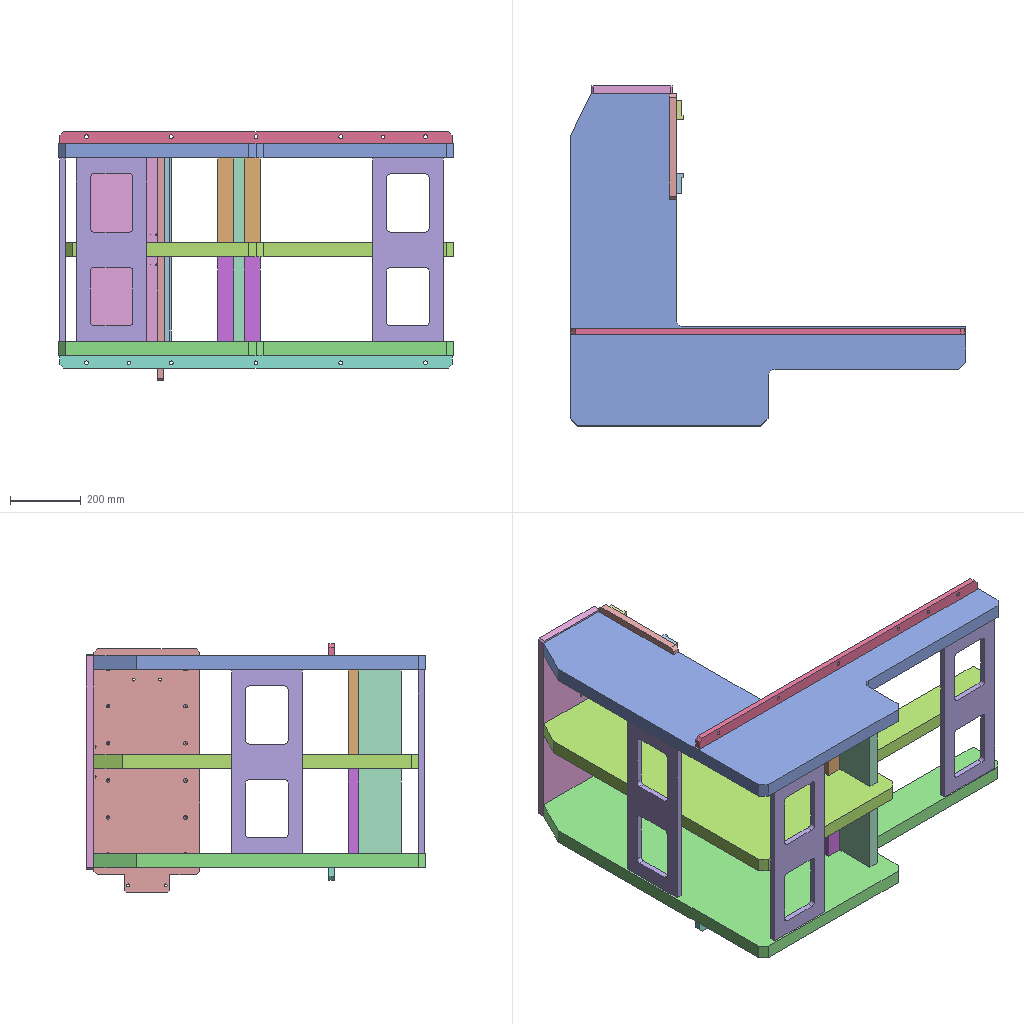Assembly | SolidWorks | 9 different items | 16 placed | box 1120 x 962 x 705 mm
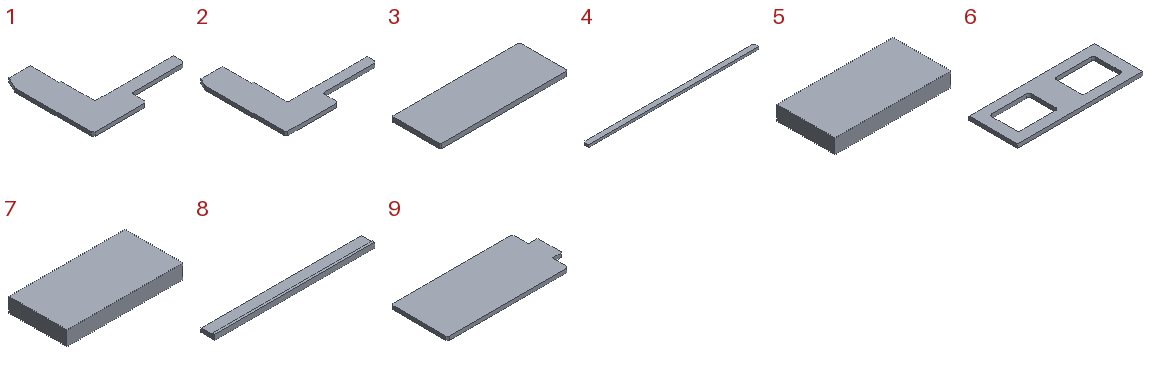Parts list (item | quantity | size | volume | features):
1 | x2 | 1120 x 940 x 40 mm | 16478867 mm3 | features Chamfer 1, Extrusion 1, Fillet 1
2 | x1 | 1099 x 919 x 40 mm | 14868507 mm3 | features Chamfer 1, Extrusion 1, Fillet 1
3 | x1 | 610 x 230 x 22 mm | 3085500 mm3 | features Chamfer 1, Extrusion 1
4 | x2 | 1110 x 35 x 16 mm | 620000 mm3 | features Chamfer 1, Extrusion 1
5 | x2 | 240 x 120 x 30 mm | 864000 mm3 | features Extrusion 1
6 | x3 | 520 x 200 x 16 mm | 1033147 mm3 | features Extrusion 1
7 | x2 | 240 x 120 x 30 mm | 864000 mm3 | features Extrusion 1
8 | x2 | 630 x 55 x 20 mm | 551250 mm3 | features Extrusion 1
9 | x1 | 690 x 300 x 20 mm | 3963509 mm3 | features Chamfer 2, Extrusion 1, Fillet 1
Mates (type | each side: item.copy, entity, surface, feature):
DistanceDim | 1.1 face plane | 2.1 face plane | 2 times
DistanceDim | 2.1 face plane | 1.2 face plane | 2 times
Coincident | 2.1 face plane | 6.1 face plane Boss-Extrude1
Coincident | 1.2 face plane | 6.1 face plane Boss-Extrude1
DistanceDim | 6.1 face plane Boss-Extrude1 | 1.2 face plane
Coincident | 6.1 face plane Boss-Extrude1 | 1.1 face plane
DistanceDim | 1.2 face plane | 2.1 face plane
Parallel | 2.1 face plane | 1.1 face plane
Coincident | 1.2 face plane | 4.1 face plane
DistanceDim | 1.2 face plane | 4.1 face plane
Coincident | 4.2 face plane | 1.1 face plane
DistanceDim | 4.2 face plane | 1.1 face plane | 2 times
DistanceDim | 4.1 face plane | 1.2 face plane
DistanceDim | 3.1 face plane | 1.2 face plane
Coincident | 3.1 edge | 1.1 edge
Coincident | 3.1 face plane | 1.1 face plane
DistanceDim | 9.1 face plane | 1.2 face plane
Coincident | 9.1 face plane | 1.2 face plane
DistanceDim | 6.2 face plane Boss-Extrude1 | 1.2 face plane
Coincident | 1.1 face plane | 6.2 face plane Boss-Extrude1
Coincident | 2.1 face plane | 6.2 face plane Boss-Extrude1
DistanceDim | 5.1 face plane | 1.2 face plane | 2 times
Coincident | 1.2 face plane | assembly plane
Parallel | 2.1 face plane | 5.1 face plane
Parallel | 1.2 face plane | 6.1 face plane Boss-Extrude1
Coincident | 2.1 face plane | assembly plane
Parallel | 9.1 face plane | 8.1 face plane | 2 times
Coincident | 9.1 face plane | 8.1 face plane
Coincident | 9.1 face plane | 8.2 face plane
DistanceDim | 9.1 face plane | 3.1 face plane
Parallel | 9.1 face plane | 8.2 face plane
DistanceDim | 9.1 face plane | 8.2 face plane
DistanceDim | 9.1 face plane | 8.1 face plane
DistanceDim | 8.2 face plane | 9.1 face plane
DistanceDim | 8.1 face plane | 9.1 face plane
Coincident | 2.1 face plane | 6.3 face plane Boss-Extrude1
DistanceDim | 6.3 face plane Boss-Extrude1 | 2.1 face plane
DistanceDim | 5.1 face plane | 2.1 face plane
DistanceDim | 5.2 face plane | 1.1 face plane | 2 times
Coincident | 5.2 face plane | 7.1 face plane Boss-Extrude1
Coincident | 1.1 face plane | 7.1 face plane Boss-Extrude1
Coincident | 1.2 face plane | 7.2 face plane Boss-Extrude1
Coincident | 5.1 face plane | 7.2 face plane Boss-Extrude1
Coincident | 2.1 face plane | 5.2 face plane
DistanceDim | 7.2 face plane Boss-Extrude1 | 5.1 face plane
DistanceDim | 7.1 face plane Boss-Extrude1 | 5.2 face plane